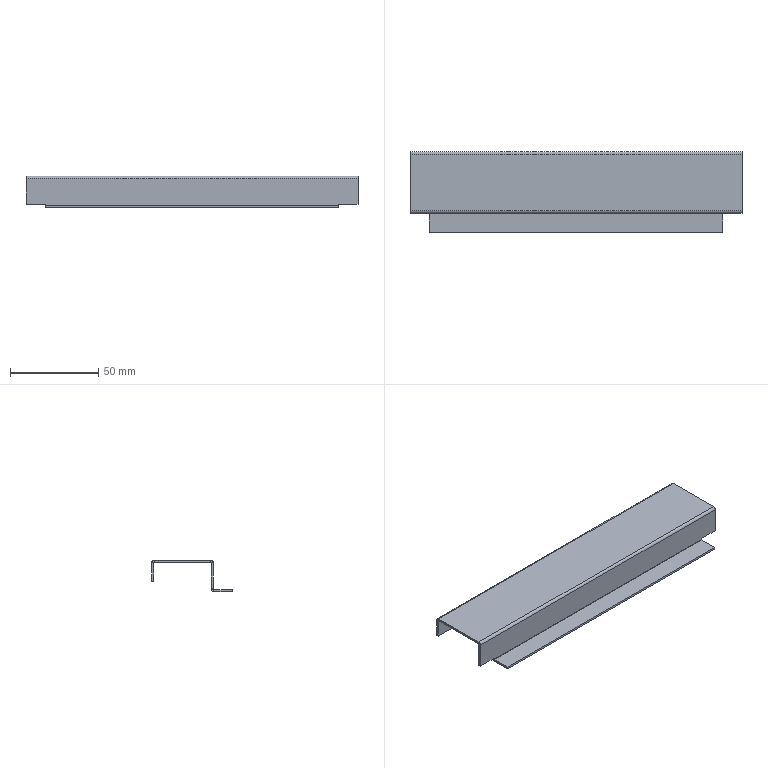Part | SolidWorks | features EdgeFlange 3, FlatPattern 1, ICE 1, SMBaseFlange 1, SheetMetal 1 | 1 solid | 34 faces | box 188 x 45.8 x 18 mm | volume 15998 mm3 | plane 28 | cylinder 6 | commonest cylinder face diameters 0.4 x3 2.8 x3
STEP:
#1=CARTESIAN_POINT('',(176.105,21.967,-16.));
#2=VERTEX_POINT('',#1);
#3=CARTESIAN_POINT('',(176.105,21.967,-16.6));
#4=VERTEX_POINT('',#3);
#5=CARTESIAN_POINT('',(176.105,21.967,-18.));
#6=DIRECTION('',(0.,0.,-1.));
#7=VECTOR('',#6,1000.);
#8=LINE('',#5,#7);
#9=EDGE_CURVE('',#2,#4,#8,.T.);
#10=ORIENTED_EDGE('',*,*,#9,.F.);
#11=CARTESIAN_POINT('',(187.105,21.967,-16.));
#12=VERTEX_POINT('',#11);
#13=CARTESIAN_POINT('',(187.105,21.967,-16.));
#14=DIRECTION('',(-1.,0.,0.));
#15=VECTOR('',#14,1000.);
#16=LINE('',#13,#15);
#17=EDGE_CURVE('',#12,#2,#16,.T.);
#18=ORIENTED_EDGE('',*,*,#17,.F.);
#19=CARTESIAN_POINT('',(187.105,21.967,-1.4));
#20=VERTEX_POINT('',#19);
#21=CARTESIAN_POINT('',(187.105,21.967,-18.));
#22=DIRECTION('',(0.,0.,-1.));
#23=VECTOR('',#22,1000.);
#24=LINE('',#21,#23);
#25=EDGE_CURVE('',#20,#12,#24,.T.);
#26=ORIENTED_EDGE('',*,*,#25,.F.);
#27=CARTESIAN_POINT('',(-0.8947,21.967,-1.4));
#28=VERTEX_POINT('',#27);
#29=CARTESIAN_POINT('',(0.,21.967,-1.4));
#30=DIRECTION('',(-1.,0.,0.));
#31=VECTOR('',#30,1000.);
#32=LINE('',#29,#31);
#33=EDGE_CURVE('',#20,#28,#32,.T.);
#34=ORIENTED_EDGE('',*,*,#33,.T.);
#35=CARTESIAN_POINT('',(-0.8947,21.967,-16.));
#36=VERTEX_POINT('',#35);
#37=CARTESIAN_POINT('',(-0.8947,21.967,-1.2));
#38=DIRECTION('',(0.,0.,1.));
#39=VECTOR('',#38,1000.);
#40=LINE('',#37,#39);
#41=EDGE_CURVE('',#36,#28,#40,.T.);
#42=ORIENTED_EDGE('',*,*,#41,.F.);
#43=CARTESIAN_POINT('',(10.105,21.967,-16.));
#44=VERTEX_POINT('',#43);
#45=CARTESIAN_POINT('',(0.,21.967,-16.));
#46=DIRECTION('',(-1.,0.,0.));
#47=VECTOR('',#46,1000.);
#48=LINE('',#45,#47);
#49=EDGE_CURVE('',#44,#36,#48,.T.);
#50=ORIENTED_EDGE('',*,*,#49,.F.);
#51=CARTESIAN_POINT('',(10.105,21.967,-16.6));
#52=VERTEX_POINT('',#51);
#53=CARTESIAN_POINT('',(10.105,21.967,0.));
#54=DIRECTION('',(0.,0.,1.));
#55=VECTOR('',#54,1000.);
#56=LINE('',#53,#55);
#57=EDGE_CURVE('',#52,#44,#56,.T.);
#58=ORIENTED_EDGE('',*,*,#57,.F.);
#59=CARTESIAN_POINT('',(176.105,21.967,-16.6));
#60=DIRECTION('',(-1.,0.,0.));
#61=VECTOR('',#60,1000.);
#62=LINE('',#59,#61);
#63=EDGE_CURVE('',#4,#52,#62,.T.);
#64=ORIENTED_EDGE('',*,*,#63,.F.);
#65=EDGE_LOOP('',(#10,#18,#26,#34,#42,#50,#58,#64));
#66=FACE_OUTER_BOUND('',#65,.T.);
#67=CARTESIAN_POINT('',(0.,21.967,0.));
#68=DIRECTION('',(0.,-1.,0.));
#69=DIRECTION('',(0.,0.,-1.));
#70=AXIS2_PLACEMENT_3D('',#67,#68,#69);
#71=PLANE('',#70);
#72=ADVANCED_FACE('',(#66),#71,.T.);
#73=CARTESIAN_POINT('',(187.105,23.167,-16.));
#74=VERTEX_POINT('',#73);
#75=CARTESIAN_POINT('',(176.105,23.167,-16.));
#76=VERTEX_POINT('',#75);
#77=CARTESIAN_POINT('',(0.,23.167,-16.));
#78=DIRECTION('',(-1.,0.,0.));
#79=VECTOR('',#78,1000.);
#80=LINE('',#77,#79);
#81=EDGE_CURVE('',#74,#76,#80,.T.);
#82=ORIENTED_EDGE('',*,*,#81,.T.);
#83=CARTESIAN_POINT('',(176.105,23.167,-16.6));
#84=VERTEX_POINT('',#83);
#85=CARTESIAN_POINT('',(176.105,23.167,0.));
#86=DIRECTION('',(0.,0.,-1.));
#87=VECTOR('',#86,1000.);
#88=LINE('',#85,#87);
#89=EDGE_CURVE('',#76,#84,#88,.T.);
#90=ORIENTED_EDGE('',*,*,#89,.T.);
#91=CARTESIAN_POINT('',(10.105,23.167,-16.6));
#92=VERTEX_POINT('',#91);
#93=CARTESIAN_POINT('',(176.105,23.167,-16.6));
#94=DIRECTION('',(-1.,0.,0.));
#95=VECTOR('',#94,1000.);
#96=LINE('',#93,#95);
#97=EDGE_CURVE('',#84,#92,#96,.T.);
#98=ORIENTED_EDGE('',*,*,#97,.T.);
#99=CARTESIAN_POINT('',(10.105,23.167,-16.));
#100=VERTEX_POINT('',#99);
#101=CARTESIAN_POINT('',(10.105,23.167,-18.));
#102=DIRECTION('',(0.,0.,1.));
#103=VECTOR('',#102,1000.);
#104=LINE('',#101,#103);
#105=EDGE_CURVE('',#92,#100,#104,.T.);
#106=ORIENTED_EDGE('',*,*,#105,.T.);
#107=CARTESIAN_POINT('',(-0.8947,23.167,-16.));
#108=VERTEX_POINT('',#107);
#109=CARTESIAN_POINT('',(-0.8947,23.167,-16.));
#110=DIRECTION('',(-1.,0.,0.));
#111=VECTOR('',#110,1000.);
#112=LINE('',#109,#111);
#113=EDGE_CURVE('',#100,#108,#112,.T.);
#114=ORIENTED_EDGE('',*,*,#113,.T.);
#115=CARTESIAN_POINT('',(-0.8947,23.167,-1.4));
#116=VERTEX_POINT('',#115);
#117=CARTESIAN_POINT('',(-0.8947,23.167,0.));
#118=DIRECTION('',(0.,0.,1.));
#119=VECTOR('',#118,1000.);
#120=LINE('',#117,#119);
#121=EDGE_CURVE('',#108,#116,#120,.T.);
#122=ORIENTED_EDGE('',*,*,#121,.T.);
#123=CARTESIAN_POINT('',(187.105,23.167,-1.4));
#124=VERTEX_POINT('',#123);
#125=CARTESIAN_POINT('',(187.105,23.167,-1.4));
#126=DIRECTION('',(-1.,0.,0.));
#127=VECTOR('',#126,1000.);
#128=LINE('',#125,#127);
#129=EDGE_CURVE('',#124,#116,#128,.T.);
#130=ORIENTED_EDGE('',*,*,#129,.F.);
#131=CARTESIAN_POINT('',(187.105,23.167,0.));
#132=DIRECTION('',(0.,0.,-1.));
#133=VECTOR('',#132,1000.);
#134=LINE('',#131,#133);
#135=EDGE_CURVE('',#124,#74,#134,.T.);
#136=ORIENTED_EDGE('',*,*,#135,.T.);
#137=EDGE_LOOP('',(#82,#90,#98,#106,#114,#122,#130,#136));
#138=FACE_OUTER_BOUND('',#137,.T.);
#139=CARTESIAN_POINT('',(0.,23.167,0.));
#140=DIRECTION('',(0.,-1.,0.));
#141=DIRECTION('',(0.,0.,-1.));
#142=AXIS2_PLACEMENT_3D('',#139,#140,#141);
#143=PLANE('',#142);
#144=ADVANCED_FACE('',(#138),#143,.F.);
#145=ORIENTED_EDGE('',*,*,#25,.T.);
#146=CARTESIAN_POINT('',(187.105,21.967,-16.));
#147=DIRECTION('',(0.,1.,0.));
#148=VECTOR('',#147,1000.);
#149=LINE('',#146,#148);
#150=EDGE_CURVE('',#12,#74,#149,.T.);
#151=ORIENTED_EDGE('',*,*,#150,.T.);
#152=ORIENTED_EDGE('',*,*,#135,.F.);
#153=CARTESIAN_POINT('',(187.105,21.967,-1.4));
#154=DIRECTION('',(0.,-1.,0.));
#155=VECTOR('',#154,1000.);
#156=LINE('',#153,#155);
#157=EDGE_CURVE('',#124,#20,#156,.T.);
#158=ORIENTED_EDGE('',*,*,#157,.T.);
#159=EDGE_LOOP('',(#145,#151,#152,#158));
#160=FACE_OUTER_BOUND('',#159,.T.);
#161=CARTESIAN_POINT('',(187.105,21.967,-18.));
#162=DIRECTION('',(1.,0.,0.));
#163=DIRECTION('',(0.,0.,-1.));
#164=AXIS2_PLACEMENT_3D('',#161,#162,#163);
#165=PLANE('',#164);
#166=ADVANCED_FACE('',(#160),#165,.T.);
#167=ORIENTED_EDGE('',*,*,#121,.F.);
#168=CARTESIAN_POINT('',(-0.8947,23.167,-16.));
#169=DIRECTION('',(0.,-1.,0.));
#170=VECTOR('',#169,1000.);
#171=LINE('',#168,#170);
#172=EDGE_CURVE('',#108,#36,#171,.T.);
#173=ORIENTED_EDGE('',*,*,#172,.T.);
#174=ORIENTED_EDGE('',*,*,#41,.T.);
#175=CARTESIAN_POINT('',(-0.8947,23.167,-1.4));
#176=DIRECTION('',(0.,-1.,0.));
#177=VECTOR('',#176,1000.);
#178=LINE('',#175,#177);
#179=EDGE_CURVE('',#116,#28,#178,.T.);
#180=ORIENTED_EDGE('',*,*,#179,.F.);
#181=EDGE_LOOP('',(#167,#173,#174,#180));
#182=FACE_OUTER_BOUND('',#181,.T.);
#183=CARTESIAN_POINT('',(-0.8947,21.967,-1.2));
#184=DIRECTION('',(-1.,0.,0.));
#185=DIRECTION('',(0.,0.,1.));
#186=AXIS2_PLACEMENT_3D('',#183,#184,#185);
#187=PLANE('',#186);
#188=ADVANCED_FACE('',(#182),#187,.T.);
#189=CARTESIAN_POINT('',(187.105,23.367,-1.2));
#190=VERTEX_POINT('',#189);
#191=CARTESIAN_POINT('',(187.105,55.567,-1.2));
#192=VERTEX_POINT('',#191);
#193=CARTESIAN_POINT('',(187.105,21.967,-1.2));
#194=DIRECTION('',(0.,1.,0.));
#195=VECTOR('',#194,1000.);
#196=LINE('',#193,#195);
#197=EDGE_CURVE('',#190,#192,#196,.T.);
#198=ORIENTED_EDGE('',*,*,#197,.F.);
#199=CARTESIAN_POINT('',(-0.8947,23.367,-1.2));
#200=VERTEX_POINT('',#199);
#201=CARTESIAN_POINT('',(-0.8947,23.367,-1.2));
#202=DIRECTION('',(1.,0.,0.));
#203=VECTOR('',#202,1000.);
#204=LINE('',#201,#203);
#205=EDGE_CURVE('',#200,#190,#204,.T.);
#206=ORIENTED_EDGE('',*,*,#205,.F.);
#207=CARTESIAN_POINT('',(-0.8947,55.567,-1.2));
#208=VERTEX_POINT('',#207);
#209=CARTESIAN_POINT('',(-0.8947,21.967,-1.2));
#210=DIRECTION('',(0.,-1.,0.));
#211=VECTOR('',#210,1000.);
#212=LINE('',#209,#211);
#213=EDGE_CURVE('',#208,#200,#212,.T.);
#214=ORIENTED_EDGE('',*,*,#213,.F.);
#215=CARTESIAN_POINT('',(187.105,55.567,-1.2));
#216=DIRECTION('',(-1.,0.,0.));
#217=VECTOR('',#216,1000.);
#218=LINE('',#215,#217);
#219=EDGE_CURVE('',#192,#208,#218,.T.);
#220=ORIENTED_EDGE('',*,*,#219,.F.);
#221=EDGE_LOOP('',(#198,#206,#214,#220));
#222=FACE_OUTER_BOUND('',#221,.T.);
#223=CARTESIAN_POINT('',(0.,0.,-1.2));
#224=DIRECTION('',(0.,0.,-1.));
#225=DIRECTION('',(-1.,0.,0.));
#226=AXIS2_PLACEMENT_3D('',#223,#224,#225);
#227=PLANE('',#226);
#228=ADVANCED_FACE('',(#222),#227,.T.);
#229=CARTESIAN_POINT('',(-0.8947,23.367,0.));
#230=VERTEX_POINT('',#229);
#231=CARTESIAN_POINT('',(187.105,23.367,0.));
#232=VERTEX_POINT('',#231);
#233=CARTESIAN_POINT('',(-0.8947,23.367,0.));
#234=DIRECTION('',(1.,0.,0.));
#235=VECTOR('',#234,1000.);
#236=LINE('',#233,#235);
#237=EDGE_CURVE('',#230,#232,#236,.T.);
#238=ORIENTED_EDGE('',*,*,#237,.T.);
#239=CARTESIAN_POINT('',(187.105,55.567,0.));
#240=VERTEX_POINT('',#239);
#241=CARTESIAN_POINT('',(187.105,21.967,0.));
#242=DIRECTION('',(0.,1.,0.));
#243=VECTOR('',#242,1000.);
#244=LINE('',#241,#243);
#245=EDGE_CURVE('',#232,#240,#244,.T.);
#246=ORIENTED_EDGE('',*,*,#245,.T.);
#247=CARTESIAN_POINT('',(-0.8947,55.567,0.));
#248=VERTEX_POINT('',#247);
#249=CARTESIAN_POINT('',(187.105,55.567,0.));
#250=DIRECTION('',(-1.,0.,0.));
#251=VECTOR('',#250,1000.);
#252=LINE('',#249,#251);
#253=EDGE_CURVE('',#240,#248,#252,.T.);
#254=ORIENTED_EDGE('',*,*,#253,.T.);
#255=CARTESIAN_POINT('',(-0.8947,21.967,0.));
#256=DIRECTION('',(0.,-1.,0.));
#257=VECTOR('',#256,1000.);
#258=LINE('',#255,#257);
#259=EDGE_CURVE('',#248,#230,#258,.T.);
#260=ORIENTED_EDGE('',*,*,#259,.T.);
#261=EDGE_LOOP('',(#238,#246,#254,#260));
#262=FACE_OUTER_BOUND('',#261,.T.);
#263=CARTESIAN_POINT('',(0.,0.,0.));
#264=DIRECTION('',(0.,0.,-1.));
#265=DIRECTION('',(-1.,0.,0.));
#266=AXIS2_PLACEMENT_3D('',#263,#264,#265);
#267=PLANE('',#266);
#268=ADVANCED_FACE('',(#262),#267,.F.);
#269=ORIENTED_EDGE('',*,*,#213,.T.);
#270=CARTESIAN_POINT('',(-0.8947,23.367,-1.2));
#271=DIRECTION('',(0.,0.,1.));
#272=VECTOR('',#271,1000.);
#273=LINE('',#270,#272);
#274=EDGE_CURVE('',#200,#230,#273,.T.);
#275=ORIENTED_EDGE('',*,*,#274,.T.);
#276=ORIENTED_EDGE('',*,*,#259,.F.);
#277=CARTESIAN_POINT('',(-0.8947,55.567,-1.2));
#278=DIRECTION('',(0.,0.,1.));
#279=VECTOR('',#278,1000.);
#280=LINE('',#277,#279);
#281=EDGE_CURVE('',#208,#248,#280,.T.);
#282=ORIENTED_EDGE('',*,*,#281,.F.);
#283=EDGE_LOOP('',(#269,#275,#276,#282));
#284=FACE_OUTER_BOUND('',#283,.T.);
#285=CARTESIAN_POINT('',(-0.8947,21.967,-1.2));
#286=DIRECTION('',(-1.,0.,0.));
#287=DIRECTION('',(0.,0.,1.));
#288=AXIS2_PLACEMENT_3D('',#285,#286,#287);
#289=PLANE('',#288);
#290=ADVANCED_FACE('',(#284),#289,.T.);
#291=CARTESIAN_POINT('',(187.105,23.367,-1.2));
#292=DIRECTION('',(0.,0.,1.));
#293=VECTOR('',#292,1000.);
#294=LINE('',#291,#293);
#295=EDGE_CURVE('',#190,#232,#294,.T.);
#296=ORIENTED_EDGE('',*,*,#295,.F.);
#297=ORIENTED_EDGE('',*,*,#197,.T.);
#298=CARTESIAN_POINT('',(187.105,55.567,-1.2));
#299=DIRECTION('',(0.,0.,1.));
#300=VECTOR('',#299,1000.);
#301=LINE('',#298,#300);
#302=EDGE_CURVE('',#192,#240,#301,.T.);
#303=ORIENTED_EDGE('',*,*,#302,.T.);
#304=ORIENTED_EDGE('',*,*,#245,.F.);
#305=EDGE_LOOP('',(#296,#297,#303,#304));
#306=FACE_OUTER_BOUND('',#305,.T.);
#307=CARTESIAN_POINT('',(187.105,21.967,-1.2));
#308=DIRECTION('',(1.,0.,0.));
#309=DIRECTION('',(0.,0.,-1.));
#310=AXIS2_PLACEMENT_3D('',#307,#308,#309);
#311=PLANE('',#310);
#312=ADVANCED_FACE('',(#306),#311,.T.);
#313=CARTESIAN_POINT('',(-0.8947,55.767,-1.4));
#314=VERTEX_POINT('',#313);
#315=CARTESIAN_POINT('',(-0.8947,56.967,-1.4));
#316=VERTEX_POINT('',#315);
#317=CARTESIAN_POINT('',(-0.8947,56.967,-1.4));
#318=DIRECTION('',(0.,1.,0.));
#319=VECTOR('',#318,1000.);
#320=LINE('',#317,#319);
#321=EDGE_CURVE('',#314,#316,#320,.T.);
#322=ORIENTED_EDGE('',*,*,#321,.F.);
#323=CARTESIAN_POINT('',(-0.8947,55.567,-1.4));
#324=DIRECTION('',(-1.,0.,0.));
#325=DIRECTION('',(0.,0.,-1.));
#326=AXIS2_PLACEMENT_3D('',#323,#324,#325);
#327=CIRCLE('',#326,0.2);
#328=EDGE_CURVE('',#208,#314,#327,.T.);
#329=ORIENTED_EDGE('',*,*,#328,.F.);
#330=ORIENTED_EDGE('',*,*,#281,.T.);
#331=CARTESIAN_POINT('',(-0.8947,55.567,-1.4));
#332=DIRECTION('',(-1.,0.,0.));
#333=DIRECTION('',(0.,0.,-1.));
#334=AXIS2_PLACEMENT_3D('',#331,#332,#333);
#335=CIRCLE('',#334,1.4);
#336=EDGE_CURVE('',#248,#316,#335,.T.);
#337=ORIENTED_EDGE('',*,*,#336,.T.);
#338=EDGE_LOOP('',(#322,#329,#330,#337));
#339=FACE_OUTER_BOUND('',#338,.T.);
#340=CARTESIAN_POINT('',(-0.8947,55.567,-1.4));
#341=DIRECTION('',(-1.,0.,0.));
#342=DIRECTION('',(0.,0.,1.));
#343=AXIS2_PLACEMENT_3D('',#340,#341,#342);
#344=PLANE('',#343);
#345=ADVANCED_FACE('',(#339),#344,.T.);
#346=CARTESIAN_POINT('',(187.105,55.767,-1.4));
#347=VERTEX_POINT('',#346);
#348=CARTESIAN_POINT('',(187.105,55.567,-1.4));
#349=DIRECTION('',(1.,0.,0.));
#350=DIRECTION('',(0.,0.,-1.));
#351=AXIS2_PLACEMENT_3D('',#348,#349,#350);
#352=CIRCLE('',#351,0.2);
#353=EDGE_CURVE('',#347,#192,#352,.T.);
#354=ORIENTED_EDGE('',*,*,#353,.F.);
#355=CARTESIAN_POINT('',(187.105,56.967,-1.4));
#356=VERTEX_POINT('',#355);
#357=CARTESIAN_POINT('',(187.105,55.767,-1.4));
#358=DIRECTION('',(0.,1.,0.));
#359=VECTOR('',#358,1000.);
#360=LINE('',#357,#359);
#361=EDGE_CURVE('',#347,#356,#360,.T.);
#362=ORIENTED_EDGE('',*,*,#361,.T.);
#363=CARTESIAN_POINT('',(187.105,55.567,-1.4));
#364=DIRECTION('',(1.,0.,0.));
#365=DIRECTION('',(0.,0.,-1.));
#366=AXIS2_PLACEMENT_3D('',#363,#364,#365);
#367=CIRCLE('',#366,1.4);
#368=EDGE_CURVE('',#356,#240,#367,.T.);
#369=ORIENTED_EDGE('',*,*,#368,.T.);
#370=ORIENTED_EDGE('',*,*,#302,.F.);
#371=EDGE_LOOP('',(#354,#362,#369,#370));
#372=FACE_OUTER_BOUND('',#371,.T.);
#373=CARTESIAN_POINT('',(187.105,55.567,-1.4));
#374=DIRECTION('',(-1.,0.,0.));
#375=DIRECTION('',(0.,0.,1.));
#376=AXIS2_PLACEMENT_3D('',#373,#374,#375);
#377=PLANE('',#376);
#378=ADVANCED_FACE('',(#372),#377,.F.);
#379=ORIENTED_EDGE('',*,*,#253,.F.);
#380=ORIENTED_EDGE('',*,*,#368,.F.);
#381=CARTESIAN_POINT('',(0.,56.967,-1.4));
#382=DIRECTION('',(1.,0.,0.));
#383=VECTOR('',#382,1000.);
#384=LINE('',#381,#383);
#385=EDGE_CURVE('',#316,#356,#384,.T.);
#386=ORIENTED_EDGE('',*,*,#385,.F.);
#387=ORIENTED_EDGE('',*,*,#336,.F.);
#388=EDGE_LOOP('',(#379,#380,#386,#387));
#389=FACE_OUTER_BOUND('',#388,.T.);
#390=CARTESIAN_POINT('',(187.105,55.567,-1.4));
#391=DIRECTION('',(1.,0.,0.));
#392=DIRECTION('',(0.,1.,0.));
#393=AXIS2_PLACEMENT_3D('',#390,#391,#392);
#394=CYLINDRICAL_SURFACE('',#393,1.4);
#395=ADVANCED_FACE('',(#389),#394,.T.);
#396=ORIENTED_EDGE('',*,*,#219,.T.);
#397=ORIENTED_EDGE('',*,*,#328,.T.);
#398=CARTESIAN_POINT('',(-0.8947,55.767,-1.4));
#399=DIRECTION('',(1.,0.,0.));
#400=VECTOR('',#399,1000.);
#401=LINE('',#398,#400);
#402=EDGE_CURVE('',#314,#347,#401,.T.);
#403=ORIENTED_EDGE('',*,*,#402,.T.);
#404=ORIENTED_EDGE('',*,*,#353,.T.);
#405=EDGE_LOOP('',(#396,#397,#403,#404));
#406=FACE_OUTER_BOUND('',#405,.T.);
#407=CARTESIAN_POINT('',(187.105,55.567,-1.4));
#408=DIRECTION('',(1.,0.,0.));
#409=DIRECTION('',(0.,1.,0.));
#410=AXIS2_PLACEMENT_3D('',#407,#408,#409);
#411=CYLINDRICAL_SURFACE('',#410,0.2);
#412=ADVANCED_FACE('',(#406),#411,.F.);
#413=CARTESIAN_POINT('',(187.105,56.967,-12.));
#414=VERTEX_POINT('',#413);
#415=CARTESIAN_POINT('',(187.105,56.967,-1.2));
#416=DIRECTION('',(0.,0.,1.));
#417=VECTOR('',#416,1000.);
#418=LINE('',#415,#417);
#419=EDGE_CURVE('',#414,#356,#418,.T.);
#420=ORIENTED_EDGE('',*,*,#419,.T.);
#421=ORIENTED_EDGE('',*,*,#361,.F.);
#422=CARTESIAN_POINT('',(187.105,55.767,-12.));
#423=VERTEX_POINT('',#422);
#424=CARTESIAN_POINT('',(187.105,55.767,0.));
#425=DIRECTION('',(0.,0.,1.));
#426=VECTOR('',#425,1000.);
#427=LINE('',#424,#426);
#428=EDGE_CURVE('',#423,#347,#427,.T.);
#429=ORIENTED_EDGE('',*,*,#428,.F.);
#430=CARTESIAN_POINT('',(187.105,56.967,-12.));
#431=DIRECTION('',(0.,-1.,0.));
#432=VECTOR('',#431,1000.);
#433=LINE('',#430,#432);
#434=EDGE_CURVE('',#414,#423,#433,.T.);
#435=ORIENTED_EDGE('',*,*,#434,.F.);
#436=EDGE_LOOP('',(#420,#421,#429,#435));
#437=FACE_OUTER_BOUND('',#436,.T.);
#438=CARTESIAN_POINT('',(187.105,56.967,-1.2));
#439=DIRECTION('',(1.,0.,0.));
#440=DIRECTION('',(0.,0.,-1.));
#441=AXIS2_PLACEMENT_3D('',#438,#439,#440);
#442=PLANE('',#441);
#443=ADVANCED_FACE('',(#437),#442,.T.);
#444=CARTESIAN_POINT('',(-0.8947,55.767,-12.));
#445=VERTEX_POINT('',#444);
#446=CARTESIAN_POINT('',(-0.8947,55.767,0.));
#447=DIRECTION('',(0.,0.,-1.));
#448=VECTOR('',#447,1000.);
#449=LINE('',#446,#448);
#450=EDGE_CURVE('',#314,#445,#449,.T.);
#451=ORIENTED_EDGE('',*,*,#450,.F.);
#452=ORIENTED_EDGE('',*,*,#321,.T.);
#453=CARTESIAN_POINT('',(-0.8947,56.967,-12.));
#454=VERTEX_POINT('',#453);
#455=CARTESIAN_POINT('',(-0.8947,56.967,-12.));
#456=DIRECTION('',(0.,0.,-1.));
#457=VECTOR('',#456,1000.);
#458=LINE('',#455,#457);
#459=EDGE_CURVE('',#316,#454,#458,.T.);
#460=ORIENTED_EDGE('',*,*,#459,.T.);
#461=CARTESIAN_POINT('',(-0.8947,56.967,-12.));
#462=DIRECTION('',(0.,-1.,0.));
#463=VECTOR('',#462,1000.);
#464=LINE('',#461,#463);
#465=EDGE_CURVE('',#454,#445,#464,.T.);
#466=ORIENTED_EDGE('',*,*,#465,.T.);
#467=EDGE_LOOP('',(#451,#452,#460,#466));
#468=FACE_OUTER_BOUND('',#467,.T.);
#469=CARTESIAN_POINT('',(-0.8947,56.967,-12.));
#470=DIRECTION('',(-1.,0.,0.));
#471=DIRECTION('',(0.,0.,1.));
#472=AXIS2_PLACEMENT_3D('',#469,#470,#471);
#473=PLANE('',#472);
#474=ADVANCED_FACE('',(#468),#473,.T.);
#475=ORIENTED_EDGE('',*,*,#459,.F.);
#476=ORIENTED_EDGE('',*,*,#385,.T.);
#477=ORIENTED_EDGE('',*,*,#419,.F.);
#478=CARTESIAN_POINT('',(187.105,56.967,-12.));
#479=DIRECTION('',(1.,0.,0.));
#480=VECTOR('',#479,1000.);
#481=LINE('',#478,#480);
#482=EDGE_CURVE('',#454,#414,#481,.T.);
#483=ORIENTED_EDGE('',*,*,#482,.F.);
#484=EDGE_LOOP('',(#475,#476,#477,#483));
#485=FACE_OUTER_BOUND('',#484,.T.);
#486=CARTESIAN_POINT('',(0.,56.967,0.));
#487=DIRECTION('',(0.,1.,0.));
#488=DIRECTION('',(0.,0.,1.));
#489=AXIS2_PLACEMENT_3D('',#486,#487,#488);
#490=PLANE('',#489);
#491=ADVANCED_FACE('',(#485),#490,.T.);
#492=ORIENTED_EDGE('',*,*,#402,.F.);
#493=ORIENTED_EDGE('',*,*,#450,.T.);
#494=CARTESIAN_POINT('',(0.,55.767,-12.));
#495=DIRECTION('',(1.,0.,0.));
#496=VECTOR('',#495,1000.);
#497=LINE('',#494,#496);
#498=EDGE_CURVE('',#445,#423,#497,.T.);
#499=ORIENTED_EDGE('',*,*,#498,.T.);
#500=ORIENTED_EDGE('',*,*,#428,.T.);
#501=EDGE_LOOP('',(#492,#493,#499,#500));
#502=FACE_OUTER_BOUND('',#501,.T.);
#503=CARTESIAN_POINT('',(0.,55.767,0.));
#504=DIRECTION('',(0.,1.,0.));
#505=DIRECTION('',(0.,0.,1.));
#506=AXIS2_PLACEMENT_3D('',#503,#504,#505);
#507=PLANE('',#506);
#508=ADVANCED_FACE('',(#502),#507,.F.);
#509=ORIENTED_EDGE('',*,*,#498,.F.);
#510=ORIENTED_EDGE('',*,*,#465,.F.);
#511=ORIENTED_EDGE('',*,*,#482,.T.);
#512=ORIENTED_EDGE('',*,*,#434,.T.);
#513=EDGE_LOOP('',(#509,#510,#511,#512));
#514=FACE_OUTER_BOUND('',#513,.T.);
#515=CARTESIAN_POINT('',(187.105,56.967,-12.));
#516=DIRECTION('',(0.,0.,-1.));
#517=DIRECTION('',(0.,1.,0.));
#518=AXIS2_PLACEMENT_3D('',#515,#516,#517);
#519=PLANE('',#518);
#520=ADVANCED_FACE('',(#514),#519,.T.);
#521=ORIENTED_EDGE('',*,*,#157,.F.);
#522=CARTESIAN_POINT('',(187.105,23.367,-1.4));
#523=DIRECTION('',(1.,0.,0.));
#524=DIRECTION('',(0.,0.,1.));
#525=AXIS2_PLACEMENT_3D('',#522,#523,#524);
#526=CIRCLE('',#525,0.2);
#527=EDGE_CURVE('',#190,#124,#526,.T.);
#528=ORIENTED_EDGE('',*,*,#527,.F.);
#529=ORIENTED_EDGE('',*,*,#295,.T.);
#530=CARTESIAN_POINT('',(187.105,23.367,-1.4));
#531=DIRECTION('',(1.,0.,0.));
#532=DIRECTION('',(0.,0.,1.));
#533=AXIS2_PLACEMENT_3D('',#530,#531,#532);
#534=CIRCLE('',#533,1.4);
#535=EDGE_CURVE('',#232,#20,#534,.T.);
#536=ORIENTED_EDGE('',*,*,#535,.T.);
#537=EDGE_LOOP('',(#521,#528,#529,#536));
#538=FACE_OUTER_BOUND('',#537,.T.);
#539=CARTESIAN_POINT('',(187.105,23.367,-1.4));
#540=DIRECTION('',(1.,0.,0.));
#541=DIRECTION('',(0.,0.,-1.));
#542=AXIS2_PLACEMENT_3D('',#539,#540,#541);
#543=PLANE('',#542);
#544=ADVANCED_FACE('',(#538),#543,.T.);
#545=CARTESIAN_POINT('',(-0.8947,23.367,-1.4));
#546=DIRECTION('',(-1.,0.,0.));
#547=DIRECTION('',(0.,0.,1.));
#548=AXIS2_PLACEMENT_3D('',#545,#546,#547);
#549=CIRCLE('',#548,0.2);
#550=EDGE_CURVE('',#116,#200,#549,.T.);
#551=ORIENTED_EDGE('',*,*,#550,.F.);
#552=ORIENTED_EDGE('',*,*,#179,.T.);
#553=CARTESIAN_POINT('',(-0.8947,23.367,-1.4));
#554=DIRECTION('',(-1.,0.,0.));
#555=DIRECTION('',(0.,0.,1.));
#556=AXIS2_PLACEMENT_3D('',#553,#554,#555);
#557=CIRCLE('',#556,1.4);
#558=EDGE_CURVE('',#28,#230,#557,.T.);
#559=ORIENTED_EDGE('',*,*,#558,.T.);
#560=ORIENTED_EDGE('',*,*,#274,.F.);
#561=EDGE_LOOP('',(#551,#552,#559,#560));
#562=FACE_OUTER_BOUND('',#561,.T.);
#563=CARTESIAN_POINT('',(-0.8947,23.367,-1.4));
#564=DIRECTION('',(1.,0.,0.));
#565=DIRECTION('',(0.,0.,-1.));
#566=AXIS2_PLACEMENT_3D('',#563,#564,#565);
#567=PLANE('',#566);
#568=ADVANCED_FACE('',(#562),#567,.F.);
#569=ORIENTED_EDGE('',*,*,#237,.F.);
#570=ORIENTED_EDGE('',*,*,#558,.F.);
#571=ORIENTED_EDGE('',*,*,#33,.F.);
#572=ORIENTED_EDGE('',*,*,#535,.F.);
#573=EDGE_LOOP('',(#569,#570,#571,#572));
#574=FACE_OUTER_BOUND('',#573,.T.);
#575=CARTESIAN_POINT('',(-0.8947,23.367,-1.4));
#576=DIRECTION('',(-1.,0.,0.));
#577=DIRECTION('',(0.,-1.,0.));
#578=AXIS2_PLACEMENT_3D('',#575,#576,#577);
#579=CYLINDRICAL_SURFACE('',#578,1.4);
#580=ADVANCED_FACE('',(#574),#579,.T.);
#581=ORIENTED_EDGE('',*,*,#205,.T.);
#582=ORIENTED_EDGE('',*,*,#527,.T.);
#583=ORIENTED_EDGE('',*,*,#129,.T.);
#584=ORIENTED_EDGE('',*,*,#550,.T.);
#585=EDGE_LOOP('',(#581,#582,#583,#584));
#586=FACE_OUTER_BOUND('',#585,.T.);
#587=CARTESIAN_POINT('',(-0.8947,23.367,-1.4));
#588=DIRECTION('',(-1.,0.,0.));
#589=DIRECTION('',(0.,-1.,0.));
#590=AXIS2_PLACEMENT_3D('',#587,#588,#589);
#591=CYLINDRICAL_SURFACE('',#590,0.2);
#592=ADVANCED_FACE('',(#586),#591,.F.);
#593=CARTESIAN_POINT('',(10.105,21.767,-16.8));
#594=VERTEX_POINT('',#593);
#595=CARTESIAN_POINT('',(10.105,21.767,-16.6));
#596=DIRECTION('',(-1.,0.,0.));
#597=DIRECTION('',(0.,0.,-1.));
#598=AXIS2_PLACEMENT_3D('',#595,#596,#597);
#599=CIRCLE('',#598,0.2);
#600=EDGE_CURVE('',#52,#594,#599,.T.);
#601=ORIENTED_EDGE('',*,*,#600,.F.);
#602=CARTESIAN_POINT('',(10.105,23.167,-16.6));
#603=DIRECTION('',(0.,-1.,0.));
#604=VECTOR('',#603,1000.);
#605=LINE('',#602,#604);
#606=EDGE_CURVE('',#92,#52,#605,.T.);
#607=ORIENTED_EDGE('',*,*,#606,.F.);
#608=CARTESIAN_POINT('',(10.105,21.767,-18.));
#609=VERTEX_POINT('',#608);
#610=CARTESIAN_POINT('',(10.105,21.767,-16.6));
#611=DIRECTION('',(-1.,0.,0.));
#612=DIRECTION('',(0.,0.,-1.));
#613=AXIS2_PLACEMENT_3D('',#610,#611,#612);
#614=CIRCLE('',#613,1.4);
#615=EDGE_CURVE('',#92,#609,#614,.T.);
#616=ORIENTED_EDGE('',*,*,#615,.T.);
#617=CARTESIAN_POINT('',(10.105,21.767,-18.));
#618=DIRECTION('',(0.,0.,-1.));
#619=VECTOR('',#618,1000.);
#620=LINE('',#617,#619);
#621=EDGE_CURVE('',#594,#609,#620,.T.);
#622=ORIENTED_EDGE('',*,*,#621,.F.);
#623=EDGE_LOOP('',(#601,#607,#616,#622));
#624=FACE_OUTER_BOUND('',#623,.T.);
#625=CARTESIAN_POINT('',(10.105,21.767,-16.6));
#626=DIRECTION('',(-1.,0.,0.));
#627=DIRECTION('',(0.,0.,1.));
#628=AXIS2_PLACEMENT_3D('',#625,#626,#627);
#629=PLANE('',#628);
#630=ADVANCED_FACE('',(#624),#629,.T.);
#631=CARTESIAN_POINT('',(176.105,21.767,-16.8));
#632=VERTEX_POINT('',#631);
#633=CARTESIAN_POINT('',(176.105,21.767,-18.));
#634=VERTEX_POINT('',#633);
#635=CARTESIAN_POINT('',(176.105,21.767,-16.8));
#636=DIRECTION('',(0.,0.,-1.));
#637=VECTOR('',#636,1000.);
#638=LINE('',#635,#637);
#639=EDGE_CURVE('',#632,#634,#638,.T.);
#640=ORIENTED_EDGE('',*,*,#639,.T.);
#641=CARTESIAN_POINT('',(176.105,21.767,-16.6));
#642=DIRECTION('',(1.,0.,0.));
#643=DIRECTION('',(0.,0.,-1.));
#644=AXIS2_PLACEMENT_3D('',#641,#642,#643);
#645=CIRCLE('',#644,1.4);
#646=EDGE_CURVE('',#634,#84,#645,.T.);
#647=ORIENTED_EDGE('',*,*,#646,.T.);
#648=CARTESIAN_POINT('',(176.105,21.967,-16.6));
#649=DIRECTION('',(0.,1.,0.));
#650=VECTOR('',#649,1000.);
#651=LINE('',#648,#650);
#652=EDGE_CURVE('',#4,#84,#651,.T.);
#653=ORIENTED_EDGE('',*,*,#652,.F.);
#654=CARTESIAN_POINT('',(176.105,21.767,-16.6));
#655=DIRECTION('',(1.,0.,0.));
#656=DIRECTION('',(0.,0.,-1.));
#657=AXIS2_PLACEMENT_3D('',#654,#655,#656);
#658=CIRCLE('',#657,0.2);
#659=EDGE_CURVE('',#632,#4,#658,.T.);
#660=ORIENTED_EDGE('',*,*,#659,.F.);
#661=EDGE_LOOP('',(#640,#647,#653,#660));
#662=FACE_OUTER_BOUND('',#661,.T.);
#663=CARTESIAN_POINT('',(176.105,21.767,-16.6));
#664=DIRECTION('',(-1.,0.,0.));
#665=DIRECTION('',(0.,0.,1.));
#666=AXIS2_PLACEMENT_3D('',#663,#664,#665);
#667=PLANE('',#666);
#668=ADVANCED_FACE('',(#662),#667,.F.);
#669=ORIENTED_EDGE('',*,*,#97,.F.);
#670=ORIENTED_EDGE('',*,*,#646,.F.);
#671=CARTESIAN_POINT('',(0.,21.767,-18.));
#672=DIRECTION('',(1.,0.,0.));
#673=VECTOR('',#672,1000.);
#674=LINE('',#671,#673);
#675=EDGE_CURVE('',#609,#634,#674,.T.);
#676=ORIENTED_EDGE('',*,*,#675,.F.);
#677=ORIENTED_EDGE('',*,*,#615,.F.);
#678=EDGE_LOOP('',(#669,#670,#676,#677));
#679=FACE_OUTER_BOUND('',#678,.T.);
#680=CARTESIAN_POINT('',(176.105,21.767,-16.6));
#681=DIRECTION('',(1.,0.,0.));
#682=DIRECTION('',(0.,0.,-1.));
#683=AXIS2_PLACEMENT_3D('',#680,#681,#682);
#684=CYLINDRICAL_SURFACE('',#683,1.4);
#685=ADVANCED_FACE('',(#679),#684,.T.);
#686=ORIENTED_EDGE('',*,*,#63,.T.);
#687=ORIENTED_EDGE('',*,*,#600,.T.);
#688=CARTESIAN_POINT('',(10.105,21.767,-16.8));
#689=DIRECTION('',(1.,0.,0.));
#690=VECTOR('',#689,1000.);
#691=LINE('',#688,#690);
#692=EDGE_CURVE('',#594,#632,#691,.T.);
#693=ORIENTED_EDGE('',*,*,#692,.T.);
#694=ORIENTED_EDGE('',*,*,#659,.T.);
#695=EDGE_LOOP('',(#686,#687,#693,#694));
#696=FACE_OUTER_BOUND('',#695,.T.);
#697=CARTESIAN_POINT('',(176.105,21.767,-16.6));
#698=DIRECTION('',(1.,0.,0.));
#699=DIRECTION('',(0.,0.,-1.));
#700=AXIS2_PLACEMENT_3D('',#697,#698,#699);
#701=CYLINDRICAL_SURFACE('',#700,0.2);
#702=ADVANCED_FACE('',(#696),#701,.F.);
#703=CARTESIAN_POINT('',(176.105,11.167,-18.));
#704=VERTEX_POINT('',#703);
#705=CARTESIAN_POINT('',(176.105,21.967,-18.));
#706=DIRECTION('',(0.,1.,0.));
#707=VECTOR('',#706,1000.);
#708=LINE('',#705,#707);
#709=EDGE_CURVE('',#704,#634,#708,.T.);
#710=ORIENTED_EDGE('',*,*,#709,.T.);
#711=ORIENTED_EDGE('',*,*,#639,.F.);
#712=CARTESIAN_POINT('',(176.105,11.167,-16.8));
#713=VERTEX_POINT('',#712);
#714=CARTESIAN_POINT('',(176.105,0.,-16.8));
#715=DIRECTION('',(0.,1.,0.));
#716=VECTOR('',#715,1000.);
#717=LINE('',#714,#716);
#718=EDGE_CURVE('',#713,#632,#717,.T.);
#719=ORIENTED_EDGE('',*,*,#718,.F.);
#720=CARTESIAN_POINT('',(176.105,11.167,-18.));
#721=DIRECTION('',(0.,0.,1.));
#722=VECTOR('',#721,1000.);
#723=LINE('',#720,#722);
#724=EDGE_CURVE('',#704,#713,#723,.T.);
#725=ORIENTED_EDGE('',*,*,#724,.F.);
#726=EDGE_LOOP('',(#710,#711,#719,#725));
#727=FACE_OUTER_BOUND('',#726,.T.);
#728=CARTESIAN_POINT('',(176.105,21.967,-18.));
#729=DIRECTION('',(1.,0.,0.));
#730=DIRECTION('',(0.,0.,-1.));
#731=AXIS2_PLACEMENT_3D('',#728,#729,#730);
#732=PLANE('',#731);
#733=ADVANCED_FACE('',(#727),#732,.T.);
#734=CARTESIAN_POINT('',(10.105,11.167,-16.8));
#735=VERTEX_POINT('',#734);
#736=CARTESIAN_POINT('',(10.105,0.,-16.8));
#737=DIRECTION('',(0.,-1.,0.));
#738=VECTOR('',#737,1000.);
#739=LINE('',#736,#738);
#740=EDGE_CURVE('',#594,#735,#739,.T.);
#741=ORIENTED_EDGE('',*,*,#740,.F.);
#742=ORIENTED_EDGE('',*,*,#621,.T.);
#743=CARTESIAN_POINT('',(10.105,11.167,-18.));
#744=VERTEX_POINT('',#743);
#745=CARTESIAN_POINT('',(10.105,11.167,-18.));
#746=DIRECTION('',(0.,-1.,0.));
#747=VECTOR('',#746,1000.);
#748=LINE('',#745,#747);
#749=EDGE_CURVE('',#609,#744,#748,.T.);
#750=ORIENTED_EDGE('',*,*,#749,.T.);
#751=CARTESIAN_POINT('',(10.105,11.167,-18.));
#752=DIRECTION('',(0.,0.,1.));
#753=VECTOR('',#752,1000.);
#754=LINE('',#751,#753);
#755=EDGE_CURVE('',#744,#735,#754,.T.);
#756=ORIENTED_EDGE('',*,*,#755,.T.);
#757=EDGE_LOOP('',(#741,#742,#750,#756));
#758=FACE_OUTER_BOUND('',#757,.T.);
#759=CARTESIAN_POINT('',(10.105,11.167,-18.));
#760=DIRECTION('',(-1.,0.,0.));
#761=DIRECTION('',(0.,-1.,0.));
#762=AXIS2_PLACEMENT_3D('',#759,#760,#761);
#763=PLANE('',#762);
#764=ADVANCED_FACE('',(#758),#763,.T.);
#765=ORIENTED_EDGE('',*,*,#749,.F.);
#766=ORIENTED_EDGE('',*,*,#675,.T.);
#767=ORIENTED_EDGE('',*,*,#709,.F.);
#768=CARTESIAN_POINT('',(176.105,11.167,-18.));
#769=DIRECTION('',(1.,0.,0.));
#770=VECTOR('',#769,1000.);
#771=LINE('',#768,#770);
#772=EDGE_CURVE('',#744,#704,#771,.T.);
#773=ORIENTED_EDGE('',*,*,#772,.F.);
#774=EDGE_LOOP('',(#765,#766,#767,#773));
#775=FACE_OUTER_BOUND('',#774,.T.);
#776=CARTESIAN_POINT('',(0.,0.,-18.));
#777=DIRECTION('',(0.,0.,-1.));
#778=DIRECTION('',(-1.,0.,0.));
#779=AXIS2_PLACEMENT_3D('',#776,#777,#778);
#780=PLANE('',#779);
#781=ADVANCED_FACE('',(#775),#780,.T.);
#782=ORIENTED_EDGE('',*,*,#692,.F.);
#783=ORIENTED_EDGE('',*,*,#740,.T.);
#784=CARTESIAN_POINT('',(0.,11.167,-16.8));
#785=DIRECTION('',(1.,0.,0.));
#786=VECTOR('',#785,1000.);
#787=LINE('',#784,#786);
#788=EDGE_CURVE('',#735,#713,#787,.T.);
#789=ORIENTED_EDGE('',*,*,#788,.T.);
#790=ORIENTED_EDGE('',*,*,#718,.T.);
#791=EDGE_LOOP('',(#782,#783,#789,#790));
#792=FACE_OUTER_BOUND('',#791,.T.);
#793=CARTESIAN_POINT('',(0.,0.,-16.8));
#794=DIRECTION('',(0.,0.,-1.));
#795=DIRECTION('',(-1.,0.,0.));
#796=AXIS2_PLACEMENT_3D('',#793,#794,#795);
#797=PLANE('',#796);
#798=ADVANCED_FACE('',(#792),#797,.F.);
#799=ORIENTED_EDGE('',*,*,#788,.F.);
#800=ORIENTED_EDGE('',*,*,#755,.F.);
#801=ORIENTED_EDGE('',*,*,#772,.T.);
#802=ORIENTED_EDGE('',*,*,#724,.T.);
#803=EDGE_LOOP('',(#799,#800,#801,#802));
#804=FACE_OUTER_BOUND('',#803,.T.);
#805=CARTESIAN_POINT('',(176.105,11.167,-18.));
#806=DIRECTION('',(0.,-1.,0.));
#807=DIRECTION('',(0.,0.,-1.));
#808=AXIS2_PLACEMENT_3D('',#805,#806,#807);
#809=PLANE('',#808);
#810=ADVANCED_FACE('',(#804),#809,.T.);
#811=ORIENTED_EDGE('',*,*,#172,.F.);
#812=ORIENTED_EDGE('',*,*,#113,.F.);
#813=CARTESIAN_POINT('',(10.105,23.167,-16.));
#814=DIRECTION('',(0.,-1.,0.));
#815=VECTOR('',#814,1000.);
#816=LINE('',#813,#815);
#817=EDGE_CURVE('',#100,#44,#816,.T.);
#818=ORIENTED_EDGE('',*,*,#817,.T.);
#819=ORIENTED_EDGE('',*,*,#49,.T.);
#820=EDGE_LOOP('',(#811,#812,#818,#819));
#821=FACE_OUTER_BOUND('',#820,.T.);
#822=CARTESIAN_POINT('',(-0.8947,23.167,-16.));
#823=DIRECTION('',(0.,0.,1.));
#824=DIRECTION('',(-1.,0.,0.));
#825=AXIS2_PLACEMENT_3D('',#822,#823,#824);
#826=PLANE('',#825);
#827=ADVANCED_FACE('',(#821),#826,.F.);
#828=ORIENTED_EDGE('',*,*,#105,.F.);
#829=ORIENTED_EDGE('',*,*,#606,.T.);
#830=ORIENTED_EDGE('',*,*,#57,.T.);
#831=ORIENTED_EDGE('',*,*,#817,.F.);
#832=EDGE_LOOP('',(#828,#829,#830,#831));
#833=FACE_OUTER_BOUND('',#832,.T.);
#834=CARTESIAN_POINT('',(10.105,23.167,-18.));
#835=DIRECTION('',(1.,0.,0.));
#836=DIRECTION('',(0.,0.,1.));
#837=AXIS2_PLACEMENT_3D('',#834,#835,#836);
#838=PLANE('',#837);
#839=ADVANCED_FACE('',(#833),#838,.F.);
#840=ORIENTED_EDGE('',*,*,#150,.F.);
#841=ORIENTED_EDGE('',*,*,#17,.T.);
#842=CARTESIAN_POINT('',(176.105,21.967,-16.));
#843=DIRECTION('',(0.,1.,0.));
#844=VECTOR('',#843,1000.);
#845=LINE('',#842,#844);
#846=EDGE_CURVE('',#2,#76,#845,.T.);
#847=ORIENTED_EDGE('',*,*,#846,.T.);
#848=ORIENTED_EDGE('',*,*,#81,.F.);
#849=EDGE_LOOP('',(#840,#841,#847,#848));
#850=FACE_OUTER_BOUND('',#849,.T.);
#851=CARTESIAN_POINT('',(187.105,21.967,-16.));
#852=DIRECTION('',(0.,0.,1.));
#853=DIRECTION('',(-1.,0.,0.));
#854=AXIS2_PLACEMENT_3D('',#851,#852,#853);
#855=PLANE('',#854);
#856=ADVANCED_FACE('',(#850),#855,.F.);
#857=ORIENTED_EDGE('',*,*,#9,.T.);
#858=ORIENTED_EDGE('',*,*,#652,.T.);
#859=ORIENTED_EDGE('',*,*,#89,.F.);
#860=ORIENTED_EDGE('',*,*,#846,.F.);
#861=EDGE_LOOP('',(#857,#858,#859,#860));
#862=FACE_OUTER_BOUND('',#861,.T.);
#863=CARTESIAN_POINT('',(176.105,21.967,-18.));
#864=DIRECTION('',(-1.,0.,0.));
#865=DIRECTION('',(0.,0.,-1.));
#866=AXIS2_PLACEMENT_3D('',#863,#864,#865);
#867=PLANE('',#866);
#868=ADVANCED_FACE('',(#862),#867,.F.);
#869=CLOSED_SHELL('',(#72,#144,#166,#188,#228,#268,#290,#312,#345,#378,#395,#412,#443,#474,#491,#508,#520,#544,#568,#580,#592,#630,#668,#685,#702,#733,#764,#781,#798,#810,#827,#839,#856,#868));
#870=MANIFOLD_SOLID_BREP('',#869);
#871=CARTESIAN_POINT('',(0.,0.,0.));
#872=DIRECTION('',(0.,0.,1.));
#873=DIRECTION('',(1.,0.,0.));
#874=AXIS2_PLACEMENT_3D('',#871,#872,#873);
#875=(LENGTH_UNIT()NAMED_UNIT(*)SI_UNIT(.MILLI.,.METRE.));
#876=UNCERTAINTY_MEASURE_WITH_UNIT(LENGTH_MEASURE(0.00001),#875,'','');
#877=(NAMED_UNIT(*)PLANE_ANGLE_UNIT()SI_UNIT($,.RADIAN.));
#878=(NAMED_UNIT(*)SI_UNIT($,.STERADIAN.)SOLID_ANGLE_UNIT());
#879=(GEOMETRIC_REPRESENTATION_CONTEXT(3)GLOBAL_UNCERTAINTY_ASSIGNED_CONTEXT((#876))GLOBAL_UNIT_ASSIGNED_CONTEXT((#875,#877,#878))REPRESENTATION_CONTEXT('',''));
#880=ADVANCED_BREP_SHAPE_REPRESENTATION('',(#870,#874),#879);